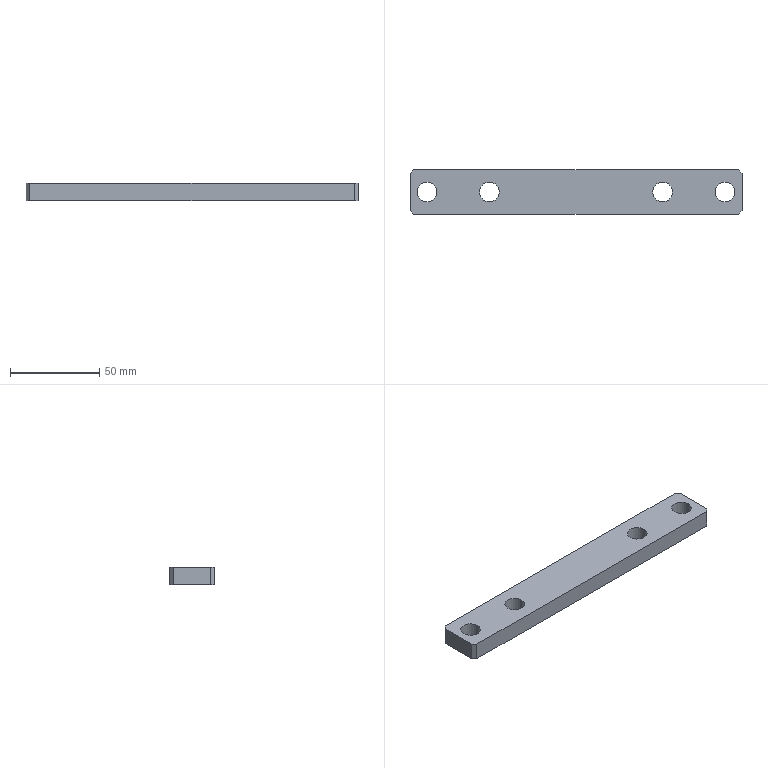Part | STEP file | Pad Plate | 1 solid | 18 faces | box 186 x 25 x 10 mm | volume 42619 mm3 | plane 10 | cylinder 8 | commonest cylinder face diameters 11 x8
STEP:
#1=CARTESIAN_POINT('',(0.,0.,0.));
#2=DIRECTION('',(0.,0.,1.));
#3=DIRECTION('',(1.,0.,0.));
#4=AXIS2_PLACEMENT_3D('',#1,#2,#3);
#5=CARTESIAN_POINT('',(89.,0.,0.));
#6=VERTEX_POINT('',#5);
#7=CARTESIAN_POINT('',(89.,0.,10.));
#8=VERTEX_POINT('',#7);
#9=CARTESIAN_POINT('',(89.,0.,-0.001));
#10=DIRECTION('',(0.,0.,1.));
#11=VECTOR('',#10,1.);
#12=LINE('',#9,#11);
#13=CARTESIAN_POINT('',(83.5,0.,-0.001));
#14=DIRECTION('',(0.,0.,1.));
#15=DIRECTION('',(1.,0.,0.));
#16=AXIS2_PLACEMENT_3D('',#13,#14,#15);
#17=CYLINDRICAL_SURFACE('',#16,5.5);
#18=CARTESIAN_POINT('',(6.283,0.));
#19=DIRECTION('',(0.,1.));
#20=VECTOR('',#19,1.);
#21=LINE('',#18,#20);
#22=(GEOMETRIC_REPRESENTATION_CONTEXT(2)PARAMETRIC_REPRESENTATION_CONTEXT()REPRESENTATION_CONTEXT('',''));
#23=DEFINITIONAL_REPRESENTATION('',(#21),#22);
#24=PCURVE('',#17,#23);
#25=CARTESIAN_POINT('',(83.5,0.,-0.001));
#26=DIRECTION('',(0.,0.,1.));
#27=DIRECTION('',(1.,0.,0.));
#28=AXIS2_PLACEMENT_3D('',#25,#26,#27);
#29=CYLINDRICAL_SURFACE('',#28,5.5);
#30=CARTESIAN_POINT('',(0.,0.));
#31=DIRECTION('',(0.,1.));
#32=VECTOR('',#31,1.);
#33=LINE('',#30,#32);
#34=(GEOMETRIC_REPRESENTATION_CONTEXT(2)PARAMETRIC_REPRESENTATION_CONTEXT()REPRESENTATION_CONTEXT('',''));
#35=DEFINITIONAL_REPRESENTATION('',(#33),#34);
#36=PCURVE('',#29,#35);
#37=SURFACE_CURVE('',#12,(#24,#36),.PCURVE_S1.);
#38=EDGE_CURVE('',#6,#8,#37,.T.);
#39=ORIENTED_EDGE('',*,*,#38,.T.);
#40=CARTESIAN_POINT('',(78.,0.,10.));
#41=VERTEX_POINT('',#40);
#42=CARTESIAN_POINT('',(83.5,0.,10.));
#43=DIRECTION('',(0.,0.,1.));
#44=DIRECTION('',(1.,0.,0.));
#45=AXIS2_PLACEMENT_3D('',#42,#43,#44);
#46=CIRCLE('',#45,5.5);
#47=CARTESIAN_POINT('',(0.,10.001));
#48=DIRECTION('',(1.,0.));
#49=VECTOR('',#48,1.);
#50=LINE('',#47,#49);
#51=(GEOMETRIC_REPRESENTATION_CONTEXT(2)PARAMETRIC_REPRESENTATION_CONTEXT()REPRESENTATION_CONTEXT('',''));
#52=DEFINITIONAL_REPRESENTATION('',(#50),#51);
#53=PCURVE('',#17,#52);
#54=CARTESIAN_POINT('',(0.,0.,10.));
#55=DIRECTION('',(0.,0.,1.));
#56=DIRECTION('',(1.,0.,0.));
#57=AXIS2_PLACEMENT_3D('',#54,#55,#56);
#58=PLANE('',#57);
#59=CARTESIAN_POINT('',(83.5,0.));
#60=DIRECTION('',(1.,0.));
#61=AXIS2_PLACEMENT_2D('',#59,#60);
#62=CIRCLE('',#61,5.5);
#63=(GEOMETRIC_REPRESENTATION_CONTEXT(2)PARAMETRIC_REPRESENTATION_CONTEXT()REPRESENTATION_CONTEXT('',''));
#64=DEFINITIONAL_REPRESENTATION('',(#62),#63);
#65=PCURVE('',#58,#64);
#66=SURFACE_CURVE('',#46,(#53,#65),.PCURVE_S1.);
#67=EDGE_CURVE('',#41,#8,#66,.T.);
#68=ORIENTED_EDGE('',*,*,#67,.F.);
#69=CARTESIAN_POINT('',(78.,0.,0.));
#70=VERTEX_POINT('',#69);
#71=CARTESIAN_POINT('',(78.,0.,-0.001));
#72=DIRECTION('',(0.,0.,1.));
#73=VECTOR('',#72,1.);
#74=LINE('',#71,#73);
#75=CARTESIAN_POINT('',(3.142,0.));
#76=DIRECTION('',(0.,1.));
#77=VECTOR('',#76,1.);
#78=LINE('',#75,#77);
#79=(GEOMETRIC_REPRESENTATION_CONTEXT(2)PARAMETRIC_REPRESENTATION_CONTEXT()REPRESENTATION_CONTEXT('',''));
#80=DEFINITIONAL_REPRESENTATION('',(#78),#79);
#81=PCURVE('',#17,#80);
#82=CARTESIAN_POINT('',(3.142,0.));
#83=DIRECTION('',(0.,1.));
#84=VECTOR('',#83,1.);
#85=LINE('',#82,#84);
#86=(GEOMETRIC_REPRESENTATION_CONTEXT(2)PARAMETRIC_REPRESENTATION_CONTEXT()REPRESENTATION_CONTEXT('',''));
#87=DEFINITIONAL_REPRESENTATION('',(#85),#86);
#88=PCURVE('',#29,#87);
#89=SURFACE_CURVE('',#74,(#81,#88),.PCURVE_S1.);
#90=EDGE_CURVE('',#70,#41,#89,.T.);
#91=ORIENTED_EDGE('',*,*,#90,.F.);
#92=CARTESIAN_POINT('',(83.5,0.,0.));
#93=DIRECTION('',(0.,0.,-1.));
#94=DIRECTION('',(1.,0.,0.));
#95=AXIS2_PLACEMENT_3D('',#92,#93,#94);
#96=CIRCLE('',#95,5.5);
#97=CARTESIAN_POINT('',(6.283,0.001));
#98=DIRECTION('',(-1.,0.));
#99=VECTOR('',#98,1.);
#100=LINE('',#97,#99);
#101=(GEOMETRIC_REPRESENTATION_CONTEXT(2)PARAMETRIC_REPRESENTATION_CONTEXT()REPRESENTATION_CONTEXT('',''));
#102=DEFINITIONAL_REPRESENTATION('',(#100),#101);
#103=PCURVE('',#17,#102);
#104=CARTESIAN_POINT('',(0.,0.,0.));
#105=DIRECTION('',(0.,0.,1.));
#106=DIRECTION('',(1.,0.,0.));
#107=AXIS2_PLACEMENT_3D('',#104,#105,#106);
#108=PLANE('',#107);
#109=CARTESIAN_POINT('',(89.,0.));
#110=CARTESIAN_POINT('',(89.,-9.526));
#111=CARTESIAN_POINT('',(80.75,-4.763));
#112=CARTESIAN_POINT('',(72.5,0.));
#113=CARTESIAN_POINT('',(80.75,4.763));
#114=CARTESIAN_POINT('',(89.,9.526));
#115=CARTESIAN_POINT('',(89.,0.));
#116=(BOUNDED_CURVE()B_SPLINE_CURVE(2,(#109,#110,#111,#112,#113,#114,#115),.UNSPECIFIED.,.T.,.F.)B_SPLINE_CURVE_WITH_KNOTS((1,2,2,2,2,1),(-2.094,0.,2.094,4.189,6.283,8.378),.UNSPECIFIED.)CURVE()GEOMETRIC_REPRESENTATION_ITEM()RATIONAL_B_SPLINE_CURVE((1.,0.5,1.,0.5,1.,0.5,1.))REPRESENTATION_ITEM(''));
#117=(GEOMETRIC_REPRESENTATION_CONTEXT(2)PARAMETRIC_REPRESENTATION_CONTEXT()REPRESENTATION_CONTEXT('',''));
#118=DEFINITIONAL_REPRESENTATION('',(#116),#117);
#119=PCURVE('',#108,#118);
#120=SURFACE_CURVE('',#96,(#103,#119),.PCURVE_S1.);
#121=EDGE_CURVE('',#6,#70,#120,.T.);
#122=ORIENTED_EDGE('',*,*,#121,.F.);
#123=EDGE_LOOP('',(#39,#68,#91,#122));
#124=FACE_BOUND('',#123,.F.);
#125=ADVANCED_FACE('',(#124),#17,.F.);
#126=CARTESIAN_POINT('',(54.,0.,0.));
#127=VERTEX_POINT('',#126);
#128=CARTESIAN_POINT('',(54.,0.,10.));
#129=VERTEX_POINT('',#128);
#130=CARTESIAN_POINT('',(54.,0.,-0.001));
#131=DIRECTION('',(0.,0.,1.));
#132=VECTOR('',#131,1.);
#133=LINE('',#130,#132);
#134=CARTESIAN_POINT('',(48.5,0.,-0.001));
#135=DIRECTION('',(0.,0.,1.));
#136=DIRECTION('',(1.,0.,0.));
#137=AXIS2_PLACEMENT_3D('',#134,#135,#136);
#138=CYLINDRICAL_SURFACE('',#137,5.5);
#139=CARTESIAN_POINT('',(6.283,0.));
#140=DIRECTION('',(0.,1.));
#141=VECTOR('',#140,1.);
#142=LINE('',#139,#141);
#143=(GEOMETRIC_REPRESENTATION_CONTEXT(2)PARAMETRIC_REPRESENTATION_CONTEXT()REPRESENTATION_CONTEXT('',''));
#144=DEFINITIONAL_REPRESENTATION('',(#142),#143);
#145=PCURVE('',#138,#144);
#146=CARTESIAN_POINT('',(48.5,0.,-0.001));
#147=DIRECTION('',(0.,0.,1.));
#148=DIRECTION('',(1.,0.,0.));
#149=AXIS2_PLACEMENT_3D('',#146,#147,#148);
#150=CYLINDRICAL_SURFACE('',#149,5.5);
#151=CARTESIAN_POINT('',(0.,0.));
#152=DIRECTION('',(0.,1.));
#153=VECTOR('',#152,1.);
#154=LINE('',#151,#153);
#155=(GEOMETRIC_REPRESENTATION_CONTEXT(2)PARAMETRIC_REPRESENTATION_CONTEXT()REPRESENTATION_CONTEXT('',''));
#156=DEFINITIONAL_REPRESENTATION('',(#154),#155);
#157=PCURVE('',#150,#156);
#158=SURFACE_CURVE('',#133,(#145,#157),.PCURVE_S1.);
#159=EDGE_CURVE('',#127,#129,#158,.T.);
#160=ORIENTED_EDGE('',*,*,#159,.T.);
#161=CARTESIAN_POINT('',(43.,0.,10.));
#162=VERTEX_POINT('',#161);
#163=CARTESIAN_POINT('',(48.5,0.,10.));
#164=DIRECTION('',(0.,0.,1.));
#165=DIRECTION('',(1.,0.,0.));
#166=AXIS2_PLACEMENT_3D('',#163,#164,#165);
#167=CIRCLE('',#166,5.5);
#168=CARTESIAN_POINT('',(0.,10.001));
#169=DIRECTION('',(1.,0.));
#170=VECTOR('',#169,1.);
#171=LINE('',#168,#170);
#172=(GEOMETRIC_REPRESENTATION_CONTEXT(2)PARAMETRIC_REPRESENTATION_CONTEXT()REPRESENTATION_CONTEXT('',''));
#173=DEFINITIONAL_REPRESENTATION('',(#171),#172);
#174=PCURVE('',#138,#173);
#175=CARTESIAN_POINT('',(48.5,0.));
#176=DIRECTION('',(1.,0.));
#177=AXIS2_PLACEMENT_2D('',#175,#176);
#178=CIRCLE('',#177,5.5);
#179=(GEOMETRIC_REPRESENTATION_CONTEXT(2)PARAMETRIC_REPRESENTATION_CONTEXT()REPRESENTATION_CONTEXT('',''));
#180=DEFINITIONAL_REPRESENTATION('',(#178),#179);
#181=PCURVE('',#58,#180);
#182=SURFACE_CURVE('',#167,(#174,#181),.PCURVE_S1.);
#183=EDGE_CURVE('',#162,#129,#182,.T.);
#184=ORIENTED_EDGE('',*,*,#183,.F.);
#185=CARTESIAN_POINT('',(43.,0.,0.));
#186=VERTEX_POINT('',#185);
#187=CARTESIAN_POINT('',(43.,0.,-0.001));
#188=DIRECTION('',(0.,0.,1.));
#189=VECTOR('',#188,1.);
#190=LINE('',#187,#189);
#191=CARTESIAN_POINT('',(3.142,0.));
#192=DIRECTION('',(0.,1.));
#193=VECTOR('',#192,1.);
#194=LINE('',#191,#193);
#195=(GEOMETRIC_REPRESENTATION_CONTEXT(2)PARAMETRIC_REPRESENTATION_CONTEXT()REPRESENTATION_CONTEXT('',''));
#196=DEFINITIONAL_REPRESENTATION('',(#194),#195);
#197=PCURVE('',#138,#196);
#198=CARTESIAN_POINT('',(3.142,0.));
#199=DIRECTION('',(0.,1.));
#200=VECTOR('',#199,1.);
#201=LINE('',#198,#200);
#202=(GEOMETRIC_REPRESENTATION_CONTEXT(2)PARAMETRIC_REPRESENTATION_CONTEXT()REPRESENTATION_CONTEXT('',''));
#203=DEFINITIONAL_REPRESENTATION('',(#201),#202);
#204=PCURVE('',#150,#203);
#205=SURFACE_CURVE('',#190,(#197,#204),.PCURVE_S1.);
#206=EDGE_CURVE('',#186,#162,#205,.T.);
#207=ORIENTED_EDGE('',*,*,#206,.F.);
#208=CARTESIAN_POINT('',(48.5,0.,0.));
#209=DIRECTION('',(0.,0.,-1.));
#210=DIRECTION('',(1.,0.,0.));
#211=AXIS2_PLACEMENT_3D('',#208,#209,#210);
#212=CIRCLE('',#211,5.5);
#213=CARTESIAN_POINT('',(6.283,0.001));
#214=DIRECTION('',(-1.,0.));
#215=VECTOR('',#214,1.);
#216=LINE('',#213,#215);
#217=(GEOMETRIC_REPRESENTATION_CONTEXT(2)PARAMETRIC_REPRESENTATION_CONTEXT()REPRESENTATION_CONTEXT('',''));
#218=DEFINITIONAL_REPRESENTATION('',(#216),#217);
#219=PCURVE('',#138,#218);
#220=CARTESIAN_POINT('',(54.,0.));
#221=CARTESIAN_POINT('',(54.,-9.526));
#222=CARTESIAN_POINT('',(45.75,-4.763));
#223=CARTESIAN_POINT('',(37.5,0.));
#224=CARTESIAN_POINT('',(45.75,4.763));
#225=CARTESIAN_POINT('',(54.,9.526));
#226=CARTESIAN_POINT('',(54.,0.));
#227=(BOUNDED_CURVE()B_SPLINE_CURVE(2,(#220,#221,#222,#223,#224,#225,#226),.UNSPECIFIED.,.T.,.F.)B_SPLINE_CURVE_WITH_KNOTS((1,2,2,2,2,1),(-2.094,0.,2.094,4.189,6.283,8.378),.UNSPECIFIED.)CURVE()GEOMETRIC_REPRESENTATION_ITEM()RATIONAL_B_SPLINE_CURVE((1.,0.5,1.,0.5,1.,0.5,1.))REPRESENTATION_ITEM(''));
#228=(GEOMETRIC_REPRESENTATION_CONTEXT(2)PARAMETRIC_REPRESENTATION_CONTEXT()REPRESENTATION_CONTEXT('',''));
#229=DEFINITIONAL_REPRESENTATION('',(#227),#228);
#230=PCURVE('',#108,#229);
#231=SURFACE_CURVE('',#212,(#219,#230),.PCURVE_S1.);
#232=EDGE_CURVE('',#127,#186,#231,.T.);
#233=ORIENTED_EDGE('',*,*,#232,.F.);
#234=EDGE_LOOP('',(#160,#184,#207,#233));
#235=FACE_BOUND('',#234,.F.);
#236=ADVANCED_FACE('',(#235),#138,.F.);
#237=CARTESIAN_POINT('',(-43.,0.,0.));
#238=VERTEX_POINT('',#237);
#239=CARTESIAN_POINT('',(-43.,0.,10.));
#240=VERTEX_POINT('',#239);
#241=CARTESIAN_POINT('',(-43.,0.,-0.001));
#242=DIRECTION('',(0.,0.,1.));
#243=VECTOR('',#242,1.);
#244=LINE('',#241,#243);
#245=CARTESIAN_POINT('',(-48.5,0.,-0.001));
#246=DIRECTION('',(0.,0.,1.));
#247=DIRECTION('',(1.,0.,0.));
#248=AXIS2_PLACEMENT_3D('',#245,#246,#247);
#249=CYLINDRICAL_SURFACE('',#248,5.5);
#250=CARTESIAN_POINT('',(6.283,0.));
#251=DIRECTION('',(0.,1.));
#252=VECTOR('',#251,1.);
#253=LINE('',#250,#252);
#254=(GEOMETRIC_REPRESENTATION_CONTEXT(2)PARAMETRIC_REPRESENTATION_CONTEXT()REPRESENTATION_CONTEXT('',''));
#255=DEFINITIONAL_REPRESENTATION('',(#253),#254);
#256=PCURVE('',#249,#255);
#257=CARTESIAN_POINT('',(-48.5,0.,-0.001));
#258=DIRECTION('',(0.,0.,1.));
#259=DIRECTION('',(1.,0.,0.));
#260=AXIS2_PLACEMENT_3D('',#257,#258,#259);
#261=CYLINDRICAL_SURFACE('',#260,5.5);
#262=CARTESIAN_POINT('',(0.,0.));
#263=DIRECTION('',(0.,1.));
#264=VECTOR('',#263,1.);
#265=LINE('',#262,#264);
#266=(GEOMETRIC_REPRESENTATION_CONTEXT(2)PARAMETRIC_REPRESENTATION_CONTEXT()REPRESENTATION_CONTEXT('',''));
#267=DEFINITIONAL_REPRESENTATION('',(#265),#266);
#268=PCURVE('',#261,#267);
#269=SURFACE_CURVE('',#244,(#256,#268),.PCURVE_S1.);
#270=EDGE_CURVE('',#238,#240,#269,.T.);
#271=ORIENTED_EDGE('',*,*,#270,.T.);
#272=CARTESIAN_POINT('',(-54.,0.,10.));
#273=VERTEX_POINT('',#272);
#274=CARTESIAN_POINT('',(-48.5,0.,10.));
#275=DIRECTION('',(0.,0.,1.));
#276=DIRECTION('',(1.,0.,0.));
#277=AXIS2_PLACEMENT_3D('',#274,#275,#276);
#278=CIRCLE('',#277,5.5);
#279=CARTESIAN_POINT('',(0.,10.001));
#280=DIRECTION('',(1.,0.));
#281=VECTOR('',#280,1.);
#282=LINE('',#279,#281);
#283=(GEOMETRIC_REPRESENTATION_CONTEXT(2)PARAMETRIC_REPRESENTATION_CONTEXT()REPRESENTATION_CONTEXT('',''));
#284=DEFINITIONAL_REPRESENTATION('',(#282),#283);
#285=PCURVE('',#249,#284);
#286=CARTESIAN_POINT('',(-48.5,0.));
#287=DIRECTION('',(1.,0.));
#288=AXIS2_PLACEMENT_2D('',#286,#287);
#289=CIRCLE('',#288,5.5);
#290=(GEOMETRIC_REPRESENTATION_CONTEXT(2)PARAMETRIC_REPRESENTATION_CONTEXT()REPRESENTATION_CONTEXT('',''));
#291=DEFINITIONAL_REPRESENTATION('',(#289),#290);
#292=PCURVE('',#58,#291);
#293=SURFACE_CURVE('',#278,(#285,#292),.PCURVE_S1.);
#294=EDGE_CURVE('',#273,#240,#293,.T.);
#295=ORIENTED_EDGE('',*,*,#294,.F.);
#296=CARTESIAN_POINT('',(-54.,0.,0.));
#297=VERTEX_POINT('',#296);
#298=CARTESIAN_POINT('',(-54.,0.,-0.001));
#299=DIRECTION('',(0.,0.,1.));
#300=VECTOR('',#299,1.);
#301=LINE('',#298,#300);
#302=CARTESIAN_POINT('',(3.142,0.));
#303=DIRECTION('',(0.,1.));
#304=VECTOR('',#303,1.);
#305=LINE('',#302,#304);
#306=(GEOMETRIC_REPRESENTATION_CONTEXT(2)PARAMETRIC_REPRESENTATION_CONTEXT()REPRESENTATION_CONTEXT('',''));
#307=DEFINITIONAL_REPRESENTATION('',(#305),#306);
#308=PCURVE('',#249,#307);
#309=CARTESIAN_POINT('',(3.142,0.));
#310=DIRECTION('',(0.,1.));
#311=VECTOR('',#310,1.);
#312=LINE('',#309,#311);
#313=(GEOMETRIC_REPRESENTATION_CONTEXT(2)PARAMETRIC_REPRESENTATION_CONTEXT()REPRESENTATION_CONTEXT('',''));
#314=DEFINITIONAL_REPRESENTATION('',(#312),#313);
#315=PCURVE('',#261,#314);
#316=SURFACE_CURVE('',#301,(#308,#315),.PCURVE_S1.);
#317=EDGE_CURVE('',#297,#273,#316,.T.);
#318=ORIENTED_EDGE('',*,*,#317,.F.);
#319=CARTESIAN_POINT('',(-48.5,0.,0.));
#320=DIRECTION('',(0.,0.,-1.));
#321=DIRECTION('',(1.,0.,0.));
#322=AXIS2_PLACEMENT_3D('',#319,#320,#321);
#323=CIRCLE('',#322,5.5);
#324=CARTESIAN_POINT('',(6.283,0.001));
#325=DIRECTION('',(-1.,0.));
#326=VECTOR('',#325,1.);
#327=LINE('',#324,#326);
#328=(GEOMETRIC_REPRESENTATION_CONTEXT(2)PARAMETRIC_REPRESENTATION_CONTEXT()REPRESENTATION_CONTEXT('',''));
#329=DEFINITIONAL_REPRESENTATION('',(#327),#328);
#330=PCURVE('',#249,#329);
#331=CARTESIAN_POINT('',(-43.,0.));
#332=CARTESIAN_POINT('',(-43.,-9.526));
#333=CARTESIAN_POINT('',(-51.25,-4.763));
#334=CARTESIAN_POINT('',(-59.5,0.));
#335=CARTESIAN_POINT('',(-51.25,4.763));
#336=CARTESIAN_POINT('',(-43.,9.526));
#337=CARTESIAN_POINT('',(-43.,0.));
#338=(BOUNDED_CURVE()B_SPLINE_CURVE(2,(#331,#332,#333,#334,#335,#336,#337),.UNSPECIFIED.,.T.,.F.)B_SPLINE_CURVE_WITH_KNOTS((1,2,2,2,2,1),(-2.094,0.,2.094,4.189,6.283,8.378),.UNSPECIFIED.)CURVE()GEOMETRIC_REPRESENTATION_ITEM()RATIONAL_B_SPLINE_CURVE((1.,0.5,1.,0.5,1.,0.5,1.))REPRESENTATION_ITEM(''));
#339=(GEOMETRIC_REPRESENTATION_CONTEXT(2)PARAMETRIC_REPRESENTATION_CONTEXT()REPRESENTATION_CONTEXT('',''));
#340=DEFINITIONAL_REPRESENTATION('',(#338),#339);
#341=PCURVE('',#108,#340);
#342=SURFACE_CURVE('',#323,(#330,#341),.PCURVE_S1.);
#343=EDGE_CURVE('',#238,#297,#342,.T.);
#344=ORIENTED_EDGE('',*,*,#343,.F.);
#345=EDGE_LOOP('',(#271,#295,#318,#344));
#346=FACE_BOUND('',#345,.F.);
#347=ADVANCED_FACE('',(#346),#249,.F.);
#348=CARTESIAN_POINT('',(-78.,0.,0.));
#349=VERTEX_POINT('',#348);
#350=CARTESIAN_POINT('',(-78.,0.,10.));
#351=VERTEX_POINT('',#350);
#352=CARTESIAN_POINT('',(-78.,0.,-0.001));
#353=DIRECTION('',(0.,0.,1.));
#354=VECTOR('',#353,1.);
#355=LINE('',#352,#354);
#356=CARTESIAN_POINT('',(-83.5,0.,-0.001));
#357=DIRECTION('',(0.,0.,1.));
#358=DIRECTION('',(1.,0.,0.));
#359=AXIS2_PLACEMENT_3D('',#356,#357,#358);
#360=CYLINDRICAL_SURFACE('',#359,5.5);
#361=CARTESIAN_POINT('',(6.283,0.));
#362=DIRECTION('',(0.,1.));
#363=VECTOR('',#362,1.);
#364=LINE('',#361,#363);
#365=(GEOMETRIC_REPRESENTATION_CONTEXT(2)PARAMETRIC_REPRESENTATION_CONTEXT()REPRESENTATION_CONTEXT('',''));
#366=DEFINITIONAL_REPRESENTATION('',(#364),#365);
#367=PCURVE('',#360,#366);
#368=CARTESIAN_POINT('',(-83.5,0.,-0.001));
#369=DIRECTION('',(0.,0.,1.));
#370=DIRECTION('',(1.,0.,0.));
#371=AXIS2_PLACEMENT_3D('',#368,#369,#370);
#372=CYLINDRICAL_SURFACE('',#371,5.5);
#373=CARTESIAN_POINT('',(0.,0.));
#374=DIRECTION('',(0.,1.));
#375=VECTOR('',#374,1.);
#376=LINE('',#373,#375);
#377=(GEOMETRIC_REPRESENTATION_CONTEXT(2)PARAMETRIC_REPRESENTATION_CONTEXT()REPRESENTATION_CONTEXT('',''));
#378=DEFINITIONAL_REPRESENTATION('',(#376),#377);
#379=PCURVE('',#372,#378);
#380=SURFACE_CURVE('',#355,(#367,#379),.PCURVE_S1.);
#381=EDGE_CURVE('',#349,#351,#380,.T.);
#382=ORIENTED_EDGE('',*,*,#381,.T.);
#383=CARTESIAN_POINT('',(-89.,0.,10.));
#384=VERTEX_POINT('',#383);
#385=CARTESIAN_POINT('',(-83.5,0.,10.));
#386=DIRECTION('',(0.,0.,1.));
#387=DIRECTION('',(1.,0.,0.));
#388=AXIS2_PLACEMENT_3D('',#385,#386,#387);
#389=CIRCLE('',#388,5.5);
#390=CARTESIAN_POINT('',(0.,10.001));
#391=DIRECTION('',(1.,0.));
#392=VECTOR('',#391,1.);
#393=LINE('',#390,#392);
#394=(GEOMETRIC_REPRESENTATION_CONTEXT(2)PARAMETRIC_REPRESENTATION_CONTEXT()REPRESENTATION_CONTEXT('',''));
#395=DEFINITIONAL_REPRESENTATION('',(#393),#394);
#396=PCURVE('',#360,#395);
#397=CARTESIAN_POINT('',(-83.5,0.));
#398=DIRECTION('',(1.,0.));
#399=AXIS2_PLACEMENT_2D('',#397,#398);
#400=CIRCLE('',#399,5.5);
#401=(GEOMETRIC_REPRESENTATION_CONTEXT(2)PARAMETRIC_REPRESENTATION_CONTEXT()REPRESENTATION_CONTEXT('',''));
#402=DEFINITIONAL_REPRESENTATION('',(#400),#401);
#403=PCURVE('',#58,#402);
#404=SURFACE_CURVE('',#389,(#396,#403),.PCURVE_S1.);
#405=EDGE_CURVE('',#384,#351,#404,.T.);
#406=ORIENTED_EDGE('',*,*,#405,.F.);
#407=CARTESIAN_POINT('',(-89.,0.,0.));
#408=VERTEX_POINT('',#407);
#409=CARTESIAN_POINT('',(-89.,0.,-0.001));
#410=DIRECTION('',(0.,0.,1.));
#411=VECTOR('',#410,1.);
#412=LINE('',#409,#411);
#413=CARTESIAN_POINT('',(3.142,0.));
#414=DIRECTION('',(0.,1.));
#415=VECTOR('',#414,1.);
#416=LINE('',#413,#415);
#417=(GEOMETRIC_REPRESENTATION_CONTEXT(2)PARAMETRIC_REPRESENTATION_CONTEXT()REPRESENTATION_CONTEXT('',''));
#418=DEFINITIONAL_REPRESENTATION('',(#416),#417);
#419=PCURVE('',#360,#418);
#420=CARTESIAN_POINT('',(3.142,0.));
#421=DIRECTION('',(0.,1.));
#422=VECTOR('',#421,1.);
#423=LINE('',#420,#422);
#424=(GEOMETRIC_REPRESENTATION_CONTEXT(2)PARAMETRIC_REPRESENTATION_CONTEXT()REPRESENTATION_CONTEXT('',''));
#425=DEFINITIONAL_REPRESENTATION('',(#423),#424);
#426=PCURVE('',#372,#425);
#427=SURFACE_CURVE('',#412,(#419,#426),.PCURVE_S1.);
#428=EDGE_CURVE('',#408,#384,#427,.T.);
#429=ORIENTED_EDGE('',*,*,#428,.F.);
#430=CARTESIAN_POINT('',(-83.5,0.,0.));
#431=DIRECTION('',(0.,0.,-1.));
#432=DIRECTION('',(1.,0.,0.));
#433=AXIS2_PLACEMENT_3D('',#430,#431,#432);
#434=CIRCLE('',#433,5.5);
#435=CARTESIAN_POINT('',(6.283,0.001));
#436=DIRECTION('',(-1.,0.));
#437=VECTOR('',#436,1.);
#438=LINE('',#435,#437);
#439=(GEOMETRIC_REPRESENTATION_CONTEXT(2)PARAMETRIC_REPRESENTATION_CONTEXT()REPRESENTATION_CONTEXT('',''));
#440=DEFINITIONAL_REPRESENTATION('',(#438),#439);
#441=PCURVE('',#360,#440);
#442=CARTESIAN_POINT('',(-78.,0.));
#443=CARTESIAN_POINT('',(-78.,-9.526));
#444=CARTESIAN_POINT('',(-86.25,-4.763));
#445=CARTESIAN_POINT('',(-94.5,0.));
#446=CARTESIAN_POINT('',(-86.25,4.763));
#447=CARTESIAN_POINT('',(-78.,9.526));
#448=CARTESIAN_POINT('',(-78.,0.));
#449=(BOUNDED_CURVE()B_SPLINE_CURVE(2,(#442,#443,#444,#445,#446,#447,#448),.UNSPECIFIED.,.T.,.F.)B_SPLINE_CURVE_WITH_KNOTS((1,2,2,2,2,1),(-2.094,0.,2.094,4.189,6.283,8.378),.UNSPECIFIED.)CURVE()GEOMETRIC_REPRESENTATION_ITEM()RATIONAL_B_SPLINE_CURVE((1.,0.5,1.,0.5,1.,0.5,1.))REPRESENTATION_ITEM(''));
#450=(GEOMETRIC_REPRESENTATION_CONTEXT(2)PARAMETRIC_REPRESENTATION_CONTEXT()REPRESENTATION_CONTEXT('',''));
#451=DEFINITIONAL_REPRESENTATION('',(#449),#450);
#452=PCURVE('',#108,#451);
#453=SURFACE_CURVE('',#434,(#441,#452),.PCURVE_S1.);
#454=EDGE_CURVE('',#349,#408,#453,.T.);
#455=ORIENTED_EDGE('',*,*,#454,.F.);
#456=EDGE_LOOP('',(#382,#406,#429,#455));
#457=FACE_BOUND('',#456,.F.);
#458=ADVANCED_FACE('',(#457),#360,.F.);
#459=CARTESIAN_POINT('',(93.,-10.5,10.));
#460=VERTEX_POINT('',#459);
#461=CARTESIAN_POINT('',(93.,10.5,10.));
#462=VERTEX_POINT('',#461);
#463=CARTESIAN_POINT('',(93.,12.5,10.));
#464=DIRECTION('',(0.,1.,0.));
#465=VECTOR('',#464,1.);
#466=LINE('',#463,#465);
#467=CARTESIAN_POINT('',(93.,12.5,10.));
#468=DIRECTION('',(-1.,0.,0.));
#469=DIRECTION('',(0.,0.,1.));
#470=AXIS2_PLACEMENT_3D('',#467,#468,#469);
#471=PLANE('',#470);
#472=CARTESIAN_POINT('',(0.,0.));
#473=DIRECTION('',(0.,1.));
#474=VECTOR('',#473,1.);
#475=LINE('',#472,#474);
#476=(GEOMETRIC_REPRESENTATION_CONTEXT(2)PARAMETRIC_REPRESENTATION_CONTEXT()REPRESENTATION_CONTEXT('',''));
#477=DEFINITIONAL_REPRESENTATION('',(#475),#476);
#478=PCURVE('',#471,#477);
#479=CARTESIAN_POINT('',(93.,12.5));
#480=DIRECTION('',(0.,1.));
#481=VECTOR('',#480,1.);
#482=LINE('',#479,#481);
#483=(GEOMETRIC_REPRESENTATION_CONTEXT(2)PARAMETRIC_REPRESENTATION_CONTEXT()REPRESENTATION_CONTEXT('',''));
#484=DEFINITIONAL_REPRESENTATION('',(#482),#483);
#485=PCURVE('',#58,#484);
#486=SURFACE_CURVE('',#466,(#478,#485),.PCURVE_S1.);
#487=EDGE_CURVE('',#460,#462,#486,.T.);
#488=ORIENTED_EDGE('',*,*,#487,.F.);
#489=CARTESIAN_POINT('',(93.,-10.5,0.));
#490=VERTEX_POINT('',#489);
#491=CARTESIAN_POINT('',(93.,-10.5,10.));
#492=DIRECTION('',(0.,0.,-1.));
#493=VECTOR('',#492,1.);
#494=LINE('',#491,#493);
#495=CARTESIAN_POINT('',(0.,-23.));
#496=DIRECTION('',(-1.,0.));
#497=VECTOR('',#496,1.);
#498=LINE('',#495,#497);
#499=(GEOMETRIC_REPRESENTATION_CONTEXT(2)PARAMETRIC_REPRESENTATION_CONTEXT()REPRESENTATION_CONTEXT('',''));
#500=DEFINITIONAL_REPRESENTATION('',(#498),#499);
#501=PCURVE('',#471,#500);
#502=CARTESIAN_POINT('',(93.,-10.5,10.));
#503=DIRECTION('',(-0.7071,0.7071,0.));
#504=DIRECTION('',(0.,0.,-1.));
#505=AXIS2_PLACEMENT_3D('',#502,#503,#504);
#506=PLANE('',#505);
#507=CARTESIAN_POINT('',(0.,0.));
#508=DIRECTION('',(1.,0.));
#509=VECTOR('',#508,1.);
#510=LINE('',#507,#509);
#511=(GEOMETRIC_REPRESENTATION_CONTEXT(2)PARAMETRIC_REPRESENTATION_CONTEXT()REPRESENTATION_CONTEXT('',''));
#512=DEFINITIONAL_REPRESENTATION('',(#510),#511);
#513=PCURVE('',#506,#512);
#514=SURFACE_CURVE('',#494,(#501,#513),.PCURVE_S1.);
#515=EDGE_CURVE('',#460,#490,#514,.T.);
#516=ORIENTED_EDGE('',*,*,#515,.T.);
#517=CARTESIAN_POINT('',(93.,10.5,0.));
#518=VERTEX_POINT('',#517);
#519=CARTESIAN_POINT('',(93.,12.5,0.));
#520=DIRECTION('',(0.,1.,0.));
#521=VECTOR('',#520,1.);
#522=LINE('',#519,#521);
#523=CARTESIAN_POINT('',(-10.,0.));
#524=DIRECTION('',(0.,1.));
#525=VECTOR('',#524,1.);
#526=LINE('',#523,#525);
#527=(GEOMETRIC_REPRESENTATION_CONTEXT(2)PARAMETRIC_REPRESENTATION_CONTEXT()REPRESENTATION_CONTEXT('',''));
#528=DEFINITIONAL_REPRESENTATION('',(#526),#527);
#529=PCURVE('',#471,#528);
#530=CARTESIAN_POINT('',(93.,12.5));
#531=DIRECTION('',(0.,1.));
#532=VECTOR('',#531,1.);
#533=LINE('',#530,#532);
#534=(GEOMETRIC_REPRESENTATION_CONTEXT(2)PARAMETRIC_REPRESENTATION_CONTEXT()REPRESENTATION_CONTEXT('',''));
#535=DEFINITIONAL_REPRESENTATION('',(#533),#534);
#536=PCURVE('',#108,#535);
#537=SURFACE_CURVE('',#522,(#529,#536),.PCURVE_S1.);
#538=EDGE_CURVE('',#490,#518,#537,.T.);
#539=ORIENTED_EDGE('',*,*,#538,.T.);
#540=CARTESIAN_POINT('',(93.,10.5,10.));
#541=DIRECTION('',(0.,0.,1.));
#542=VECTOR('',#541,1.);
#543=LINE('',#540,#542);
#544=CARTESIAN_POINT('',(0.,-2.));
#545=DIRECTION('',(1.,0.));
#546=VECTOR('',#545,1.);
#547=LINE('',#544,#546);
#548=(GEOMETRIC_REPRESENTATION_CONTEXT(2)PARAMETRIC_REPRESENTATION_CONTEXT()REPRESENTATION_CONTEXT('',''));
#549=DEFINITIONAL_REPRESENTATION('',(#547),#548);
#550=PCURVE('',#471,#549);
#551=CARTESIAN_POINT('',(91.,12.5,10.));
#552=DIRECTION('',(-0.7071,-0.7071,0.));
#553=DIRECTION('',(0.,0.,-1.));
#554=AXIS2_PLACEMENT_3D('',#551,#552,#553);
#555=PLANE('',#554);
#556=CARTESIAN_POINT('',(0.,2.828));
#557=DIRECTION('',(-1.,0.));
#558=VECTOR('',#557,1.);
#559=LINE('',#556,#558);
#560=(GEOMETRIC_REPRESENTATION_CONTEXT(2)PARAMETRIC_REPRESENTATION_CONTEXT()REPRESENTATION_CONTEXT('',''));
#561=DEFINITIONAL_REPRESENTATION('',(#559),#560);
#562=PCURVE('',#555,#561);
#563=SURFACE_CURVE('',#543,(#550,#562),.PCURVE_S1.);
#564=EDGE_CURVE('',#518,#462,#563,.T.);
#565=ORIENTED_EDGE('',*,*,#564,.T.);
#566=EDGE_LOOP('',(#488,#516,#539,#565));
#567=FACE_BOUND('',#566,.T.);
#568=ADVANCED_FACE('',(#567),#471,.F.);
#569=CARTESIAN_POINT('',(91.,12.5,10.));
#570=VERTEX_POINT('',#569);
#571=CARTESIAN_POINT('',(-91.,12.5,10.));
#572=VERTEX_POINT('',#571);
#573=CARTESIAN_POINT('',(-93.,12.5,10.));
#574=DIRECTION('',(-1.,0.,0.));
#575=VECTOR('',#574,1.);
#576=LINE('',#573,#575);
#577=CARTESIAN_POINT('',(-93.,12.5,10.));
#578=DIRECTION('',(0.,-1.,0.));
#579=DIRECTION('',(0.,0.,-1.));
#580=AXIS2_PLACEMENT_3D('',#577,#578,#579);
#581=PLANE('',#580);
#582=CARTESIAN_POINT('',(0.,0.));
#583=DIRECTION('',(0.,-1.));
#584=VECTOR('',#583,1.);
#585=LINE('',#582,#584);
#586=(GEOMETRIC_REPRESENTATION_CONTEXT(2)PARAMETRIC_REPRESENTATION_CONTEXT()REPRESENTATION_CONTEXT('',''));
#587=DEFINITIONAL_REPRESENTATION('',(#585),#586);
#588=PCURVE('',#581,#587);
#589=CARTESIAN_POINT('',(-93.,12.5));
#590=DIRECTION('',(-1.,0.));
#591=VECTOR('',#590,1.);
#592=LINE('',#589,#591);
#593=(GEOMETRIC_REPRESENTATION_CONTEXT(2)PARAMETRIC_REPRESENTATION_CONTEXT()REPRESENTATION_CONTEXT('',''));
#594=DEFINITIONAL_REPRESENTATION('',(#592),#593);
#595=PCURVE('',#58,#594);
#596=SURFACE_CURVE('',#576,(#588,#595),.PCURVE_S1.);
#597=EDGE_CURVE('',#570,#572,#596,.T.);
#598=ORIENTED_EDGE('',*,*,#597,.F.);
#599=CARTESIAN_POINT('',(91.,12.5,0.));
#600=VERTEX_POINT('',#599);
#601=CARTESIAN_POINT('',(91.,12.5,10.));
#602=DIRECTION('',(0.,0.,-1.));
#603=VECTOR('',#602,1.);
#604=LINE('',#601,#603);
#605=CARTESIAN_POINT('',(0.,184.));
#606=DIRECTION('',(1.,0.));
#607=VECTOR('',#606,1.);
#608=LINE('',#605,#607);
#609=(GEOMETRIC_REPRESENTATION_CONTEXT(2)PARAMETRIC_REPRESENTATION_CONTEXT()REPRESENTATION_CONTEXT('',''));
#610=DEFINITIONAL_REPRESENTATION('',(#608),#609);
#611=PCURVE('',#581,#610);
#612=CARTESIAN_POINT('',(0.,0.));
#613=DIRECTION('',(1.,0.));
#614=VECTOR('',#613,1.);
#615=LINE('',#612,#614);
#616=(GEOMETRIC_REPRESENTATION_CONTEXT(2)PARAMETRIC_REPRESENTATION_CONTEXT()REPRESENTATION_CONTEXT('',''));
#617=DEFINITIONAL_REPRESENTATION('',(#615),#616);
#618=PCURVE('',#555,#617);
#619=SURFACE_CURVE('',#604,(#611,#618),.PCURVE_S1.);
#620=EDGE_CURVE('',#570,#600,#619,.T.);
#621=ORIENTED_EDGE('',*,*,#620,.T.);
#622=CARTESIAN_POINT('',(-91.,12.5,0.));
#623=VERTEX_POINT('',#622);
#624=CARTESIAN_POINT('',(-93.,12.5,0.));
#625=DIRECTION('',(-1.,0.,0.));
#626=VECTOR('',#625,1.);
#627=LINE('',#624,#626);
#628=CARTESIAN_POINT('',(10.,0.));
#629=DIRECTION('',(0.,-1.));
#630=VECTOR('',#629,1.);
#631=LINE('',#628,#630);
#632=(GEOMETRIC_REPRESENTATION_CONTEXT(2)PARAMETRIC_REPRESENTATION_CONTEXT()REPRESENTATION_CONTEXT('',''));
#633=DEFINITIONAL_REPRESENTATION('',(#631),#632);
#634=PCURVE('',#581,#633);
#635=CARTESIAN_POINT('',(-93.,12.5));
#636=DIRECTION('',(-1.,0.));
#637=VECTOR('',#636,1.);
#638=LINE('',#635,#637);
#639=(GEOMETRIC_REPRESENTATION_CONTEXT(2)PARAMETRIC_REPRESENTATION_CONTEXT()REPRESENTATION_CONTEXT('',''));
#640=DEFINITIONAL_REPRESENTATION('',(#638),#639);
#641=PCURVE('',#108,#640);
#642=SURFACE_CURVE('',#627,(#634,#641),.PCURVE_S1.);
#643=EDGE_CURVE('',#600,#623,#642,.T.);
#644=ORIENTED_EDGE('',*,*,#643,.T.);
#645=CARTESIAN_POINT('',(-91.,12.5,10.));
#646=DIRECTION('',(0.,0.,1.));
#647=VECTOR('',#646,1.);
#648=LINE('',#645,#647);
#649=CARTESIAN_POINT('',(0.,2.));
#650=DIRECTION('',(-1.,0.));
#651=VECTOR('',#650,1.);
#652=LINE('',#649,#651);
#653=(GEOMETRIC_REPRESENTATION_CONTEXT(2)PARAMETRIC_REPRESENTATION_CONTEXT()REPRESENTATION_CONTEXT('',''));
#654=DEFINITIONAL_REPRESENTATION('',(#652),#653);
#655=PCURVE('',#581,#654);
#656=CARTESIAN_POINT('',(-93.,10.5,10.));
#657=DIRECTION('',(0.7071,-0.7071,0.));
#658=DIRECTION('',(0.,0.,-1.));
#659=AXIS2_PLACEMENT_3D('',#656,#657,#658);
#660=PLANE('',#659);
#661=CARTESIAN_POINT('',(0.,2.828));
#662=DIRECTION('',(-1.,0.));
#663=VECTOR('',#662,1.);
#664=LINE('',#661,#663);
#665=(GEOMETRIC_REPRESENTATION_CONTEXT(2)PARAMETRIC_REPRESENTATION_CONTEXT()REPRESENTATION_CONTEXT('',''));
#666=DEFINITIONAL_REPRESENTATION('',(#664),#665);
#667=PCURVE('',#660,#666);
#668=SURFACE_CURVE('',#648,(#655,#667),.PCURVE_S1.);
#669=EDGE_CURVE('',#623,#572,#668,.T.);
#670=ORIENTED_EDGE('',*,*,#669,.T.);
#671=EDGE_LOOP('',(#598,#621,#644,#670));
#672=FACE_BOUND('',#671,.T.);
#673=ADVANCED_FACE('',(#672),#581,.F.);
#674=CARTESIAN_POINT('',(-93.,10.5,10.));
#675=VERTEX_POINT('',#674);
#676=CARTESIAN_POINT('',(-93.,-10.5,10.));
#677=VERTEX_POINT('',#676);
#678=CARTESIAN_POINT('',(-93.,12.5,10.));
#679=DIRECTION('',(0.,-1.,0.));
#680=VECTOR('',#679,1.);
#681=LINE('',#678,#680);
#682=CARTESIAN_POINT('',(-93.,12.5,10.));
#683=DIRECTION('',(1.,0.,0.));
#684=DIRECTION('',(0.,0.,-1.));
#685=AXIS2_PLACEMENT_3D('',#682,#683,#684);
#686=PLANE('',#685);
#687=CARTESIAN_POINT('',(0.,0.));
#688=DIRECTION('',(0.,-1.));
#689=VECTOR('',#688,1.);
#690=LINE('',#687,#689);
#691=(GEOMETRIC_REPRESENTATION_CONTEXT(2)PARAMETRIC_REPRESENTATION_CONTEXT()REPRESENTATION_CONTEXT('',''));
#692=DEFINITIONAL_REPRESENTATION('',(#690),#691);
#693=PCURVE('',#686,#692);
#694=CARTESIAN_POINT('',(-93.,12.5));
#695=DIRECTION('',(0.,-1.));
#696=VECTOR('',#695,1.);
#697=LINE('',#694,#696);
#698=(GEOMETRIC_REPRESENTATION_CONTEXT(2)PARAMETRIC_REPRESENTATION_CONTEXT()REPRESENTATION_CONTEXT('',''));
#699=DEFINITIONAL_REPRESENTATION('',(#697),#698);
#700=PCURVE('',#58,#699);
#701=SURFACE_CURVE('',#681,(#693,#700),.PCURVE_S1.);
#702=EDGE_CURVE('',#675,#677,#701,.T.);
#703=ORIENTED_EDGE('',*,*,#702,.F.);
#704=CARTESIAN_POINT('',(-93.,10.5,0.));
#705=VERTEX_POINT('',#704);
#706=CARTESIAN_POINT('',(-93.,10.5,10.));
#707=DIRECTION('',(0.,0.,-1.));
#708=VECTOR('',#707,1.);
#709=LINE('',#706,#708);
#710=CARTESIAN_POINT('',(0.,-2.));
#711=DIRECTION('',(1.,0.));
#712=VECTOR('',#711,1.);
#713=LINE('',#710,#712);
#714=(GEOMETRIC_REPRESENTATION_CONTEXT(2)PARAMETRIC_REPRESENTATION_CONTEXT()REPRESENTATION_CONTEXT('',''));
#715=DEFINITIONAL_REPRESENTATION('',(#713),#714);
#716=PCURVE('',#686,#715);
#717=CARTESIAN_POINT('',(0.,0.));
#718=DIRECTION('',(1.,0.));
#719=VECTOR('',#718,1.);
#720=LINE('',#717,#719);
#721=(GEOMETRIC_REPRESENTATION_CONTEXT(2)PARAMETRIC_REPRESENTATION_CONTEXT()REPRESENTATION_CONTEXT('',''));
#722=DEFINITIONAL_REPRESENTATION('',(#720),#721);
#723=PCURVE('',#660,#722);
#724=SURFACE_CURVE('',#709,(#716,#723),.PCURVE_S1.);
#725=EDGE_CURVE('',#675,#705,#724,.T.);
#726=ORIENTED_EDGE('',*,*,#725,.T.);
#727=CARTESIAN_POINT('',(-93.,-10.5,0.));
#728=VERTEX_POINT('',#727);
#729=CARTESIAN_POINT('',(-93.,12.5,0.));
#730=DIRECTION('',(0.,-1.,0.));
#731=VECTOR('',#730,1.);
#732=LINE('',#729,#731);
#733=CARTESIAN_POINT('',(10.,0.));
#734=DIRECTION('',(0.,-1.));
#735=VECTOR('',#734,1.);
#736=LINE('',#733,#735);
#737=(GEOMETRIC_REPRESENTATION_CONTEXT(2)PARAMETRIC_REPRESENTATION_CONTEXT()REPRESENTATION_CONTEXT('',''));
#738=DEFINITIONAL_REPRESENTATION('',(#736),#737);
#739=PCURVE('',#686,#738);
#740=CARTESIAN_POINT('',(-93.,12.5));
#741=DIRECTION('',(0.,-1.));
#742=VECTOR('',#741,1.);
#743=LINE('',#740,#742);
#744=(GEOMETRIC_REPRESENTATION_CONTEXT(2)PARAMETRIC_REPRESENTATION_CONTEXT()REPRESENTATION_CONTEXT('',''));
#745=DEFINITIONAL_REPRESENTATION('',(#743),#744);
#746=PCURVE('',#108,#745);
#747=SURFACE_CURVE('',#732,(#739,#746),.PCURVE_S1.);
#748=EDGE_CURVE('',#705,#728,#747,.T.);
#749=ORIENTED_EDGE('',*,*,#748,.T.);
#750=CARTESIAN_POINT('',(-93.,-10.5,10.));
#751=DIRECTION('',(0.,0.,1.));
#752=VECTOR('',#751,1.);
#753=LINE('',#750,#752);
#754=CARTESIAN_POINT('',(0.,-23.));
#755=DIRECTION('',(-1.,0.));
#756=VECTOR('',#755,1.);
#757=LINE('',#754,#756);
#758=(GEOMETRIC_REPRESENTATION_CONTEXT(2)PARAMETRIC_REPRESENTATION_CONTEXT()REPRESENTATION_CONTEXT('',''));
#759=DEFINITIONAL_REPRESENTATION('',(#757),#758);
#760=PCURVE('',#686,#759);
#761=CARTESIAN_POINT('',(-91.,-12.5,10.));
#762=DIRECTION('',(0.7071,0.7071,0.));
#763=DIRECTION('',(0.,0.,-1.));
#764=AXIS2_PLACEMENT_3D('',#761,#762,#763);
#765=PLANE('',#764);
#766=CARTESIAN_POINT('',(0.,2.828));
#767=DIRECTION('',(-1.,0.));
#768=VECTOR('',#767,1.);
#769=LINE('',#766,#768);
#770=(GEOMETRIC_REPRESENTATION_CONTEXT(2)PARAMETRIC_REPRESENTATION_CONTEXT()REPRESENTATION_CONTEXT('',''));
#771=DEFINITIONAL_REPRESENTATION('',(#769),#770);
#772=PCURVE('',#765,#771);
#773=SURFACE_CURVE('',#753,(#760,#772),.PCURVE_S1.);
#774=EDGE_CURVE('',#728,#677,#773,.T.);
#775=ORIENTED_EDGE('',*,*,#774,.T.);
#776=EDGE_LOOP('',(#703,#726,#749,#775));
#777=FACE_BOUND('',#776,.T.);
#778=ADVANCED_FACE('',(#777),#686,.F.);
#779=CARTESIAN_POINT('',(-91.,-12.5,0.));
#780=VERTEX_POINT('',#779);
#781=CARTESIAN_POINT('',(91.,-12.5,0.));
#782=VERTEX_POINT('',#781);
#783=CARTESIAN_POINT('',(-93.,-12.5,0.));
#784=DIRECTION('',(1.,0.,0.));
#785=VECTOR('',#784,1.);
#786=LINE('',#783,#785);
#787=CARTESIAN_POINT('',(-93.,-12.5,10.));
#788=DIRECTION('',(0.,1.,0.));
#789=DIRECTION('',(0.,0.,1.));
#790=AXIS2_PLACEMENT_3D('',#787,#788,#789);
#791=PLANE('',#790);
#792=CARTESIAN_POINT('',(-10.,0.));
#793=DIRECTION('',(0.,1.));
#794=VECTOR('',#793,1.);
#795=LINE('',#792,#794);
#796=(GEOMETRIC_REPRESENTATION_CONTEXT(2)PARAMETRIC_REPRESENTATION_CONTEXT()REPRESENTATION_CONTEXT('',''));
#797=DEFINITIONAL_REPRESENTATION('',(#795),#796);
#798=PCURVE('',#791,#797);
#799=CARTESIAN_POINT('',(-93.,-12.5));
#800=DIRECTION('',(1.,0.));
#801=VECTOR('',#800,1.);
#802=LINE('',#799,#801);
#803=(GEOMETRIC_REPRESENTATION_CONTEXT(2)PARAMETRIC_REPRESENTATION_CONTEXT()REPRESENTATION_CONTEXT('',''));
#804=DEFINITIONAL_REPRESENTATION('',(#802),#803);
#805=PCURVE('',#108,#804);
#806=SURFACE_CURVE('',#786,(#798,#805),.PCURVE_S1.);
#807=EDGE_CURVE('',#780,#782,#806,.T.);
#808=ORIENTED_EDGE('',*,*,#807,.T.);
#809=CARTESIAN_POINT('',(91.,-12.5,10.));
#810=VERTEX_POINT('',#809);
#811=CARTESIAN_POINT('',(91.,-12.5,10.));
#812=DIRECTION('',(0.,0.,1.));
#813=VECTOR('',#812,1.);
#814=LINE('',#811,#813);
#815=CARTESIAN_POINT('',(0.,184.));
#816=DIRECTION('',(1.,0.));
#817=VECTOR('',#816,1.);
#818=LINE('',#815,#817);
#819=(GEOMETRIC_REPRESENTATION_CONTEXT(2)PARAMETRIC_REPRESENTATION_CONTEXT()REPRESENTATION_CONTEXT('',''));
#820=DEFINITIONAL_REPRESENTATION('',(#818),#819);
#821=PCURVE('',#791,#820);
#822=CARTESIAN_POINT('',(0.,2.828));
#823=DIRECTION('',(-1.,0.));
#824=VECTOR('',#823,1.);
#825=LINE('',#822,#824);
#826=(GEOMETRIC_REPRESENTATION_CONTEXT(2)PARAMETRIC_REPRESENTATION_CONTEXT()REPRESENTATION_CONTEXT('',''));
#827=DEFINITIONAL_REPRESENTATION('',(#825),#826);
#828=PCURVE('',#506,#827);
#829=SURFACE_CURVE('',#814,(#821,#828),.PCURVE_S1.);
#830=EDGE_CURVE('',#782,#810,#829,.T.);
#831=ORIENTED_EDGE('',*,*,#830,.T.);
#832=CARTESIAN_POINT('',(-91.,-12.5,10.));
#833=VERTEX_POINT('',#832);
#834=CARTESIAN_POINT('',(-93.,-12.5,10.));
#835=DIRECTION('',(1.,0.,0.));
#836=VECTOR('',#835,1.);
#837=LINE('',#834,#836);
#838=CARTESIAN_POINT('',(0.,0.));
#839=DIRECTION('',(0.,1.));
#840=VECTOR('',#839,1.);
#841=LINE('',#838,#840);
#842=(GEOMETRIC_REPRESENTATION_CONTEXT(2)PARAMETRIC_REPRESENTATION_CONTEXT()REPRESENTATION_CONTEXT('',''));
#843=DEFINITIONAL_REPRESENTATION('',(#841),#842);
#844=PCURVE('',#791,#843);
#845=CARTESIAN_POINT('',(-93.,-12.5));
#846=DIRECTION('',(1.,0.));
#847=VECTOR('',#846,1.);
#848=LINE('',#845,#847);
#849=(GEOMETRIC_REPRESENTATION_CONTEXT(2)PARAMETRIC_REPRESENTATION_CONTEXT()REPRESENTATION_CONTEXT('',''));
#850=DEFINITIONAL_REPRESENTATION('',(#848),#849);
#851=PCURVE('',#58,#850);
#852=SURFACE_CURVE('',#837,(#844,#851),.PCURVE_S1.);
#853=EDGE_CURVE('',#833,#810,#852,.T.);
#854=ORIENTED_EDGE('',*,*,#853,.F.);
#855=CARTESIAN_POINT('',(-91.,-12.5,10.));
#856=DIRECTION('',(0.,0.,-1.));
#857=VECTOR('',#856,1.);
#858=LINE('',#855,#857);
#859=CARTESIAN_POINT('',(0.,2.));
#860=DIRECTION('',(-1.,0.));
#861=VECTOR('',#860,1.);
#862=LINE('',#859,#861);
#863=(GEOMETRIC_REPRESENTATION_CONTEXT(2)PARAMETRIC_REPRESENTATION_CONTEXT()REPRESENTATION_CONTEXT('',''));
#864=DEFINITIONAL_REPRESENTATION('',(#862),#863);
#865=PCURVE('',#791,#864);
#866=CARTESIAN_POINT('',(0.,0.));
#867=DIRECTION('',(1.,0.));
#868=VECTOR('',#867,1.);
#869=LINE('',#866,#868);
#870=(GEOMETRIC_REPRESENTATION_CONTEXT(2)PARAMETRIC_REPRESENTATION_CONTEXT()REPRESENTATION_CONTEXT('',''));
#871=DEFINITIONAL_REPRESENTATION('',(#869),#870);
#872=PCURVE('',#765,#871);
#873=SURFACE_CURVE('',#858,(#865,#872),.PCURVE_S1.);
#874=EDGE_CURVE('',#833,#780,#873,.T.);
#875=ORIENTED_EDGE('',*,*,#874,.T.);
#876=EDGE_LOOP('',(#808,#831,#854,#875));
#877=FACE_BOUND('',#876,.T.);
#878=ADVANCED_FACE('',(#877),#791,.F.);
#879=CARTESIAN_POINT('',(83.5,0.,10.));
#880=DIRECTION('',(0.,0.,1.));
#881=DIRECTION('',(1.,0.,0.));
#882=AXIS2_PLACEMENT_3D('',#879,#880,#881);
#883=CIRCLE('',#882,5.5);
#884=CARTESIAN_POINT('',(83.5,0.));
#885=DIRECTION('',(1.,0.));
#886=AXIS2_PLACEMENT_2D('',#884,#885);
#887=CIRCLE('',#886,5.5);
#888=(GEOMETRIC_REPRESENTATION_CONTEXT(2)PARAMETRIC_REPRESENTATION_CONTEXT()REPRESENTATION_CONTEXT('',''));
#889=DEFINITIONAL_REPRESENTATION('',(#887),#888);
#890=PCURVE('',#58,#889);
#891=CARTESIAN_POINT('',(0.,10.001));
#892=DIRECTION('',(1.,0.));
#893=VECTOR('',#892,1.);
#894=LINE('',#891,#893);
#895=(GEOMETRIC_REPRESENTATION_CONTEXT(2)PARAMETRIC_REPRESENTATION_CONTEXT()REPRESENTATION_CONTEXT('',''));
#896=DEFINITIONAL_REPRESENTATION('',(#894),#895);
#897=PCURVE('',#29,#896);
#898=SURFACE_CURVE('',#883,(#890,#897),.PCURVE_S1.);
#899=EDGE_CURVE('',#8,#41,#898,.T.);
#900=ORIENTED_EDGE('',*,*,#899,.F.);
#901=ORIENTED_EDGE('',*,*,#67,.F.);
#902=EDGE_LOOP('',(#900,#901));
#903=FACE_BOUND('',#902,.T.);
#904=CARTESIAN_POINT('',(48.5,0.,10.));
#905=DIRECTION('',(0.,0.,1.));
#906=DIRECTION('',(1.,0.,0.));
#907=AXIS2_PLACEMENT_3D('',#904,#905,#906);
#908=CIRCLE('',#907,5.5);
#909=CARTESIAN_POINT('',(48.5,0.));
#910=DIRECTION('',(1.,0.));
#911=AXIS2_PLACEMENT_2D('',#909,#910);
#912=CIRCLE('',#911,5.5);
#913=(GEOMETRIC_REPRESENTATION_CONTEXT(2)PARAMETRIC_REPRESENTATION_CONTEXT()REPRESENTATION_CONTEXT('',''));
#914=DEFINITIONAL_REPRESENTATION('',(#912),#913);
#915=PCURVE('',#58,#914);
#916=CARTESIAN_POINT('',(0.,10.001));
#917=DIRECTION('',(1.,0.));
#918=VECTOR('',#917,1.);
#919=LINE('',#916,#918);
#920=(GEOMETRIC_REPRESENTATION_CONTEXT(2)PARAMETRIC_REPRESENTATION_CONTEXT()REPRESENTATION_CONTEXT('',''));
#921=DEFINITIONAL_REPRESENTATION('',(#919),#920);
#922=PCURVE('',#150,#921);
#923=SURFACE_CURVE('',#908,(#915,#922),.PCURVE_S1.);
#924=EDGE_CURVE('',#129,#162,#923,.T.);
#925=ORIENTED_EDGE('',*,*,#924,.F.);
#926=ORIENTED_EDGE('',*,*,#183,.F.);
#927=EDGE_LOOP('',(#925,#926));
#928=FACE_BOUND('',#927,.T.);
#929=CARTESIAN_POINT('',(-48.5,0.,10.));
#930=DIRECTION('',(0.,0.,1.));
#931=DIRECTION('',(1.,0.,0.));
#932=AXIS2_PLACEMENT_3D('',#929,#930,#931);
#933=CIRCLE('',#932,5.5);
#934=CARTESIAN_POINT('',(-48.5,0.));
#935=DIRECTION('',(1.,0.));
#936=AXIS2_PLACEMENT_2D('',#934,#935);
#937=CIRCLE('',#936,5.5);
#938=(GEOMETRIC_REPRESENTATION_CONTEXT(2)PARAMETRIC_REPRESENTATION_CONTEXT()REPRESENTATION_CONTEXT('',''));
#939=DEFINITIONAL_REPRESENTATION('',(#937),#938);
#940=PCURVE('',#58,#939);
#941=CARTESIAN_POINT('',(0.,10.001));
#942=DIRECTION('',(1.,0.));
#943=VECTOR('',#942,1.);
#944=LINE('',#941,#943);
#945=(GEOMETRIC_REPRESENTATION_CONTEXT(2)PARAMETRIC_REPRESENTATION_CONTEXT()REPRESENTATION_CONTEXT('',''));
#946=DEFINITIONAL_REPRESENTATION('',(#944),#945);
#947=PCURVE('',#261,#946);
#948=SURFACE_CURVE('',#933,(#940,#947),.PCURVE_S1.);
#949=EDGE_CURVE('',#240,#273,#948,.T.);
#950=ORIENTED_EDGE('',*,*,#949,.F.);
#951=ORIENTED_EDGE('',*,*,#294,.F.);
#952=EDGE_LOOP('',(#950,#951));
#953=FACE_BOUND('',#952,.T.);
#954=CARTESIAN_POINT('',(-83.5,0.,10.));
#955=DIRECTION('',(0.,0.,1.));
#956=DIRECTION('',(1.,0.,0.));
#957=AXIS2_PLACEMENT_3D('',#954,#955,#956);
#958=CIRCLE('',#957,5.5);
#959=CARTESIAN_POINT('',(-83.5,0.));
#960=DIRECTION('',(1.,0.));
#961=AXIS2_PLACEMENT_2D('',#959,#960);
#962=CIRCLE('',#961,5.5);
#963=(GEOMETRIC_REPRESENTATION_CONTEXT(2)PARAMETRIC_REPRESENTATION_CONTEXT()REPRESENTATION_CONTEXT('',''));
#964=DEFINITIONAL_REPRESENTATION('',(#962),#963);
#965=PCURVE('',#58,#964);
#966=CARTESIAN_POINT('',(0.,10.001));
#967=DIRECTION('',(1.,0.));
#968=VECTOR('',#967,1.);
#969=LINE('',#966,#968);
#970=(GEOMETRIC_REPRESENTATION_CONTEXT(2)PARAMETRIC_REPRESENTATION_CONTEXT()REPRESENTATION_CONTEXT('',''));
#971=DEFINITIONAL_REPRESENTATION('',(#969),#970);
#972=PCURVE('',#372,#971);
#973=SURFACE_CURVE('',#958,(#965,#972),.PCURVE_S1.);
#974=EDGE_CURVE('',#351,#384,#973,.T.);
#975=ORIENTED_EDGE('',*,*,#974,.F.);
#976=ORIENTED_EDGE('',*,*,#405,.F.);
#977=EDGE_LOOP('',(#975,#976));
#978=FACE_BOUND('',#977,.T.);
#979=ORIENTED_EDGE('',*,*,#853,.T.);
#980=CARTESIAN_POINT('',(51.75,-51.75,10.));
#981=DIRECTION('',(0.7071,0.7071,0.));
#982=VECTOR('',#981,1.);
#983=LINE('',#980,#982);
#984=CARTESIAN_POINT('',(51.75,-51.75));
#985=DIRECTION('',(0.7071,0.7071));
#986=VECTOR('',#985,1.);
#987=LINE('',#984,#986);
#988=(GEOMETRIC_REPRESENTATION_CONTEXT(2)PARAMETRIC_REPRESENTATION_CONTEXT()REPRESENTATION_CONTEXT('',''));
#989=DEFINITIONAL_REPRESENTATION('',(#987),#988);
#990=PCURVE('',#58,#989);
#991=CARTESIAN_POINT('',(0.,58.336));
#992=DIRECTION('',(0.,-1.));
#993=VECTOR('',#992,1.);
#994=LINE('',#991,#993);
#995=(GEOMETRIC_REPRESENTATION_CONTEXT(2)PARAMETRIC_REPRESENTATION_CONTEXT()REPRESENTATION_CONTEXT('',''));
#996=DEFINITIONAL_REPRESENTATION('',(#994),#995);
#997=PCURVE('',#506,#996);
#998=SURFACE_CURVE('',#983,(#990,#997),.PCURVE_S1.);
#999=EDGE_CURVE('',#810,#460,#998,.T.);
#1000=ORIENTED_EDGE('',*,*,#999,.T.);
#1001=ORIENTED_EDGE('',*,*,#487,.T.);
#1002=CARTESIAN_POINT('',(51.75,51.75,10.));
#1003=DIRECTION('',(-0.7071,0.7071,0.));
#1004=VECTOR('',#1003,1.);
#1005=LINE('',#1002,#1004);
#1006=CARTESIAN_POINT('',(51.75,51.75));
#1007=DIRECTION('',(-0.7071,0.7071));
#1008=VECTOR('',#1007,1.);
#1009=LINE('',#1006,#1008);
#1010=(GEOMETRIC_REPRESENTATION_CONTEXT(2)PARAMETRIC_REPRESENTATION_CONTEXT()REPRESENTATION_CONTEXT('',''));
#1011=DEFINITIONAL_REPRESENTATION('',(#1009),#1010);
#1012=PCURVE('',#58,#1011);
#1013=CARTESIAN_POINT('',(0.,-55.508));
#1014=DIRECTION('',(0.,-1.));
#1015=VECTOR('',#1014,1.);
#1016=LINE('',#1013,#1015);
#1017=(GEOMETRIC_REPRESENTATION_CONTEXT(2)PARAMETRIC_REPRESENTATION_CONTEXT()REPRESENTATION_CONTEXT('',''));
#1018=DEFINITIONAL_REPRESENTATION('',(#1016),#1017);
#1019=PCURVE('',#555,#1018);
#1020=SURFACE_CURVE('',#1005,(#1012,#1019),.PCURVE_S1.);
#1021=EDGE_CURVE('',#462,#570,#1020,.T.);
#1022=ORIENTED_EDGE('',*,*,#1021,.T.);
#1023=ORIENTED_EDGE('',*,*,#597,.T.);
#1024=CARTESIAN_POINT('',(-51.75,51.75,10.));
#1025=DIRECTION('',(-0.7071,-0.7071,0.));
#1026=VECTOR('',#1025,1.);
#1027=LINE('',#1024,#1026);
#1028=CARTESIAN_POINT('',(-51.75,51.75));
#1029=DIRECTION('',(-0.7071,-0.7071));
#1030=VECTOR('',#1029,1.);
#1031=LINE('',#1028,#1030);
#1032=(GEOMETRIC_REPRESENTATION_CONTEXT(2)PARAMETRIC_REPRESENTATION_CONTEXT()REPRESENTATION_CONTEXT('',''));
#1033=DEFINITIONAL_REPRESENTATION('',(#1031),#1032);
#1034=PCURVE('',#58,#1033);
#1035=CARTESIAN_POINT('',(0.,58.336));
#1036=DIRECTION('',(0.,-1.));
#1037=VECTOR('',#1036,1.);
#1038=LINE('',#1035,#1037);
#1039=(GEOMETRIC_REPRESENTATION_CONTEXT(2)PARAMETRIC_REPRESENTATION_CONTEXT()REPRESENTATION_CONTEXT('',''));
#1040=DEFINITIONAL_REPRESENTATION('',(#1038),#1039);
#1041=PCURVE('',#660,#1040);
#1042=SURFACE_CURVE('',#1027,(#1034,#1041),.PCURVE_S1.);
#1043=EDGE_CURVE('',#572,#675,#1042,.T.);
#1044=ORIENTED_EDGE('',*,*,#1043,.T.);
#1045=ORIENTED_EDGE('',*,*,#702,.T.);
#1046=CARTESIAN_POINT('',(-51.75,-51.75,10.));
#1047=DIRECTION('',(0.7071,-0.7071,0.));
#1048=VECTOR('',#1047,1.);
#1049=LINE('',#1046,#1048);
#1050=CARTESIAN_POINT('',(-51.75,-51.75));
#1051=DIRECTION('',(0.7071,-0.7071));
#1052=VECTOR('',#1051,1.);
#1053=LINE('',#1050,#1052);
#1054=(GEOMETRIC_REPRESENTATION_CONTEXT(2)PARAMETRIC_REPRESENTATION_CONTEXT()REPRESENTATION_CONTEXT('',''));
#1055=DEFINITIONAL_REPRESENTATION('',(#1053),#1054);
#1056=PCURVE('',#58,#1055);
#1057=CARTESIAN_POINT('',(0.,-55.508));
#1058=DIRECTION('',(0.,-1.));
#1059=VECTOR('',#1058,1.);
#1060=LINE('',#1057,#1059);
#1061=(GEOMETRIC_REPRESENTATION_CONTEXT(2)PARAMETRIC_REPRESENTATION_CONTEXT()REPRESENTATION_CONTEXT('',''));
#1062=DEFINITIONAL_REPRESENTATION('',(#1060),#1061);
#1063=PCURVE('',#765,#1062);
#1064=SURFACE_CURVE('',#1049,(#1056,#1063),.PCURVE_S1.);
#1065=EDGE_CURVE('',#677,#833,#1064,.T.);
#1066=ORIENTED_EDGE('',*,*,#1065,.T.);
#1067=EDGE_LOOP('',(#979,#1000,#1001,#1022,#1023,#1044,#1045,#1066));
#1068=FACE_BOUND('',#1067,.T.);
#1069=ADVANCED_FACE('',(#903,#928,#953,#978,#1068),#58,.T.);
#1070=ORIENTED_EDGE('',*,*,#121,.F.);
#1071=CARTESIAN_POINT('',(83.5,0.,0.));
#1072=DIRECTION('',(0.,0.,-1.));
#1073=DIRECTION('',(1.,0.,0.));
#1074=AXIS2_PLACEMENT_3D('',#1071,#1072,#1073);
#1075=CIRCLE('',#1074,5.5);
#1076=CARTESIAN_POINT('',(89.,0.));
#1077=CARTESIAN_POINT('',(89.,-9.526));
#1078=CARTESIAN_POINT('',(80.75,-4.763));
#1079=CARTESIAN_POINT('',(72.5,0.));
#1080=CARTESIAN_POINT('',(80.75,4.763));
#1081=CARTESIAN_POINT('',(89.,9.526));
#1082=CARTESIAN_POINT('',(89.,0.));
#1083=(BOUNDED_CURVE()B_SPLINE_CURVE(2,(#1076,#1077,#1078,#1079,#1080,#1081,#1082),.UNSPECIFIED.,.T.,.F.)B_SPLINE_CURVE_WITH_KNOTS((1,2,2,2,2,1),(-2.094,0.,2.094,4.189,6.283,8.378),.UNSPECIFIED.)CURVE()GEOMETRIC_REPRESENTATION_ITEM()RATIONAL_B_SPLINE_CURVE((1.,0.5,1.,0.5,1.,0.5,1.))REPRESENTATION_ITEM(''));
#1084=(GEOMETRIC_REPRESENTATION_CONTEXT(2)PARAMETRIC_REPRESENTATION_CONTEXT()REPRESENTATION_CONTEXT('',''));
#1085=DEFINITIONAL_REPRESENTATION('',(#1083),#1084);
#1086=PCURVE('',#108,#1085);
#1087=CARTESIAN_POINT('',(6.283,0.001));
#1088=DIRECTION('',(-1.,0.));
#1089=VECTOR('',#1088,1.);
#1090=LINE('',#1087,#1089);
#1091=(GEOMETRIC_REPRESENTATION_CONTEXT(2)PARAMETRIC_REPRESENTATION_CONTEXT()REPRESENTATION_CONTEXT('',''));
#1092=DEFINITIONAL_REPRESENTATION('',(#1090),#1091);
#1093=PCURVE('',#29,#1092);
#1094=SURFACE_CURVE('',#1075,(#1086,#1093),.PCURVE_S1.);
#1095=EDGE_CURVE('',#70,#6,#1094,.T.);
#1096=ORIENTED_EDGE('',*,*,#1095,.F.);
#1097=EDGE_LOOP('',(#1070,#1096));
#1098=FACE_BOUND('',#1097,.T.);
#1099=ORIENTED_EDGE('',*,*,#232,.F.);
#1100=CARTESIAN_POINT('',(48.5,0.,0.));
#1101=DIRECTION('',(0.,0.,-1.));
#1102=DIRECTION('',(1.,0.,0.));
#1103=AXIS2_PLACEMENT_3D('',#1100,#1101,#1102);
#1104=CIRCLE('',#1103,5.5);
#1105=CARTESIAN_POINT('',(54.,0.));
#1106=CARTESIAN_POINT('',(54.,-9.526));
#1107=CARTESIAN_POINT('',(45.75,-4.763));
#1108=CARTESIAN_POINT('',(37.5,0.));
#1109=CARTESIAN_POINT('',(45.75,4.763));
#1110=CARTESIAN_POINT('',(54.,9.526));
#1111=CARTESIAN_POINT('',(54.,0.));
#1112=(BOUNDED_CURVE()B_SPLINE_CURVE(2,(#1105,#1106,#1107,#1108,#1109,#1110,#1111),.UNSPECIFIED.,.T.,.F.)B_SPLINE_CURVE_WITH_KNOTS((1,2,2,2,2,1),(-2.094,0.,2.094,4.189,6.283,8.378),.UNSPECIFIED.)CURVE()GEOMETRIC_REPRESENTATION_ITEM()RATIONAL_B_SPLINE_CURVE((1.,0.5,1.,0.5,1.,0.5,1.))REPRESENTATION_ITEM(''));
#1113=(GEOMETRIC_REPRESENTATION_CONTEXT(2)PARAMETRIC_REPRESENTATION_CONTEXT()REPRESENTATION_CONTEXT('',''));
#1114=DEFINITIONAL_REPRESENTATION('',(#1112),#1113);
#1115=PCURVE('',#108,#1114);
#1116=CARTESIAN_POINT('',(6.283,0.001));
#1117=DIRECTION('',(-1.,0.));
#1118=VECTOR('',#1117,1.);
#1119=LINE('',#1116,#1118);
#1120=(GEOMETRIC_REPRESENTATION_CONTEXT(2)PARAMETRIC_REPRESENTATION_CONTEXT()REPRESENTATION_CONTEXT('',''));
#1121=DEFINITIONAL_REPRESENTATION('',(#1119),#1120);
#1122=PCURVE('',#150,#1121);
#1123=SURFACE_CURVE('',#1104,(#1115,#1122),.PCURVE_S1.);
#1124=EDGE_CURVE('',#186,#127,#1123,.T.);
#1125=ORIENTED_EDGE('',*,*,#1124,.F.);
#1126=EDGE_LOOP('',(#1099,#1125));
#1127=FACE_BOUND('',#1126,.T.);
#1128=ORIENTED_EDGE('',*,*,#343,.F.);
#1129=CARTESIAN_POINT('',(-48.5,0.,0.));
#1130=DIRECTION('',(0.,0.,-1.));
#1131=DIRECTION('',(1.,0.,0.));
#1132=AXIS2_PLACEMENT_3D('',#1129,#1130,#1131);
#1133=CIRCLE('',#1132,5.5);
#1134=CARTESIAN_POINT('',(-43.,0.));
#1135=CARTESIAN_POINT('',(-43.,-9.526));
#1136=CARTESIAN_POINT('',(-51.25,-4.763));
#1137=CARTESIAN_POINT('',(-59.5,0.));
#1138=CARTESIAN_POINT('',(-51.25,4.763));
#1139=CARTESIAN_POINT('',(-43.,9.526));
#1140=CARTESIAN_POINT('',(-43.,0.));
#1141=(BOUNDED_CURVE()B_SPLINE_CURVE(2,(#1134,#1135,#1136,#1137,#1138,#1139,#1140),.UNSPECIFIED.,.T.,.F.)B_SPLINE_CURVE_WITH_KNOTS((1,2,2,2,2,1),(-2.094,0.,2.094,4.189,6.283,8.378),.UNSPECIFIED.)CURVE()GEOMETRIC_REPRESENTATION_ITEM()RATIONAL_B_SPLINE_CURVE((1.,0.5,1.,0.5,1.,0.5,1.))REPRESENTATION_ITEM(''));
#1142=(GEOMETRIC_REPRESENTATION_CONTEXT(2)PARAMETRIC_REPRESENTATION_CONTEXT()REPRESENTATION_CONTEXT('',''));
#1143=DEFINITIONAL_REPRESENTATION('',(#1141),#1142);
#1144=PCURVE('',#108,#1143);
#1145=CARTESIAN_POINT('',(6.283,0.001));
#1146=DIRECTION('',(-1.,0.));
#1147=VECTOR('',#1146,1.);
#1148=LINE('',#1145,#1147);
#1149=(GEOMETRIC_REPRESENTATION_CONTEXT(2)PARAMETRIC_REPRESENTATION_CONTEXT()REPRESENTATION_CONTEXT('',''));
#1150=DEFINITIONAL_REPRESENTATION('',(#1148),#1149);
#1151=PCURVE('',#261,#1150);
#1152=SURFACE_CURVE('',#1133,(#1144,#1151),.PCURVE_S1.);
#1153=EDGE_CURVE('',#297,#238,#1152,.T.);
#1154=ORIENTED_EDGE('',*,*,#1153,.F.);
#1155=EDGE_LOOP('',(#1128,#1154));
#1156=FACE_BOUND('',#1155,.T.);
#1157=ORIENTED_EDGE('',*,*,#454,.F.);
#1158=CARTESIAN_POINT('',(-83.5,0.,0.));
#1159=DIRECTION('',(0.,0.,-1.));
#1160=DIRECTION('',(1.,0.,0.));
#1161=AXIS2_PLACEMENT_3D('',#1158,#1159,#1160);
#1162=CIRCLE('',#1161,5.5);
#1163=CARTESIAN_POINT('',(-78.,0.));
#1164=CARTESIAN_POINT('',(-78.,-9.526));
#1165=CARTESIAN_POINT('',(-86.25,-4.763));
#1166=CARTESIAN_POINT('',(-94.5,0.));
#1167=CARTESIAN_POINT('',(-86.25,4.763));
#1168=CARTESIAN_POINT('',(-78.,9.526));
#1169=CARTESIAN_POINT('',(-78.,0.));
#1170=(BOUNDED_CURVE()B_SPLINE_CURVE(2,(#1163,#1164,#1165,#1166,#1167,#1168,#1169),.UNSPECIFIED.,.T.,.F.)B_SPLINE_CURVE_WITH_KNOTS((1,2,2,2,2,1),(-2.094,0.,2.094,4.189,6.283,8.378),.UNSPECIFIED.)CURVE()GEOMETRIC_REPRESENTATION_ITEM()RATIONAL_B_SPLINE_CURVE((1.,0.5,1.,0.5,1.,0.5,1.))REPRESENTATION_ITEM(''));
#1171=(GEOMETRIC_REPRESENTATION_CONTEXT(2)PARAMETRIC_REPRESENTATION_CONTEXT()REPRESENTATION_CONTEXT('',''));
#1172=DEFINITIONAL_REPRESENTATION('',(#1170),#1171);
#1173=PCURVE('',#108,#1172);
#1174=CARTESIAN_POINT('',(6.283,0.001));
#1175=DIRECTION('',(-1.,0.));
#1176=VECTOR('',#1175,1.);
#1177=LINE('',#1174,#1176);
#1178=(GEOMETRIC_REPRESENTATION_CONTEXT(2)PARAMETRIC_REPRESENTATION_CONTEXT()REPRESENTATION_CONTEXT('',''));
#1179=DEFINITIONAL_REPRESENTATION('',(#1177),#1178);
#1180=PCURVE('',#372,#1179);
#1181=SURFACE_CURVE('',#1162,(#1173,#1180),.PCURVE_S1.);
#1182=EDGE_CURVE('',#408,#349,#1181,.T.);
#1183=ORIENTED_EDGE('',*,*,#1182,.F.);
#1184=EDGE_LOOP('',(#1157,#1183));
#1185=FACE_BOUND('',#1184,.T.);
#1186=ORIENTED_EDGE('',*,*,#538,.F.);
#1187=CARTESIAN_POINT('',(93.,-10.5,0.));
#1188=DIRECTION('',(-0.7071,-0.7071,0.));
#1189=VECTOR('',#1188,1.);
#1190=LINE('',#1187,#1189);
#1191=CARTESIAN_POINT('',(93.,-10.5));
#1192=DIRECTION('',(-0.7071,-0.7071));
#1193=VECTOR('',#1192,1.);
#1194=LINE('',#1191,#1193);
#1195=(GEOMETRIC_REPRESENTATION_CONTEXT(2)PARAMETRIC_REPRESENTATION_CONTEXT()REPRESENTATION_CONTEXT('',''));
#1196=DEFINITIONAL_REPRESENTATION('',(#1194),#1195);
#1197=PCURVE('',#108,#1196);
#1198=CARTESIAN_POINT('',(10.,0.));
#1199=DIRECTION('',(0.,1.));
#1200=VECTOR('',#1199,1.);
#1201=LINE('',#1198,#1200);
#1202=(GEOMETRIC_REPRESENTATION_CONTEXT(2)PARAMETRIC_REPRESENTATION_CONTEXT()REPRESENTATION_CONTEXT('',''));
#1203=DEFINITIONAL_REPRESENTATION('',(#1201),#1202);
#1204=PCURVE('',#506,#1203);
#1205=SURFACE_CURVE('',#1190,(#1197,#1204),.PCURVE_S1.);
#1206=EDGE_CURVE('',#490,#782,#1205,.T.);
#1207=ORIENTED_EDGE('',*,*,#1206,.T.);
#1208=ORIENTED_EDGE('',*,*,#807,.F.);
#1209=CARTESIAN_POINT('',(-91.,-12.5,0.));
#1210=DIRECTION('',(-0.7071,0.7071,0.));
#1211=VECTOR('',#1210,1.);
#1212=LINE('',#1209,#1211);
#1213=CARTESIAN_POINT('',(-91.,-12.5));
#1214=DIRECTION('',(-0.7071,0.7071));
#1215=VECTOR('',#1214,1.);
#1216=LINE('',#1213,#1215);
#1217=(GEOMETRIC_REPRESENTATION_CONTEXT(2)PARAMETRIC_REPRESENTATION_CONTEXT()REPRESENTATION_CONTEXT('',''));
#1218=DEFINITIONAL_REPRESENTATION('',(#1216),#1217);
#1219=PCURVE('',#108,#1218);
#1220=CARTESIAN_POINT('',(10.,0.));
#1221=DIRECTION('',(0.,1.));
#1222=VECTOR('',#1221,1.);
#1223=LINE('',#1220,#1222);
#1224=(GEOMETRIC_REPRESENTATION_CONTEXT(2)PARAMETRIC_REPRESENTATION_CONTEXT()REPRESENTATION_CONTEXT('',''));
#1225=DEFINITIONAL_REPRESENTATION('',(#1223),#1224);
#1226=PCURVE('',#765,#1225);
#1227=SURFACE_CURVE('',#1212,(#1219,#1226),.PCURVE_S1.);
#1228=EDGE_CURVE('',#780,#728,#1227,.T.);
#1229=ORIENTED_EDGE('',*,*,#1228,.T.);
#1230=ORIENTED_EDGE('',*,*,#748,.F.);
#1231=CARTESIAN_POINT('',(-93.,10.5,0.));
#1232=DIRECTION('',(0.7071,0.7071,0.));
#1233=VECTOR('',#1232,1.);
#1234=LINE('',#1231,#1233);
#1235=CARTESIAN_POINT('',(-93.,10.5));
#1236=DIRECTION('',(0.7071,0.7071));
#1237=VECTOR('',#1236,1.);
#1238=LINE('',#1235,#1237);
#1239=(GEOMETRIC_REPRESENTATION_CONTEXT(2)PARAMETRIC_REPRESENTATION_CONTEXT()REPRESENTATION_CONTEXT('',''));
#1240=DEFINITIONAL_REPRESENTATION('',(#1238),#1239);
#1241=PCURVE('',#108,#1240);
#1242=CARTESIAN_POINT('',(10.,0.));
#1243=DIRECTION('',(0.,1.));
#1244=VECTOR('',#1243,1.);
#1245=LINE('',#1242,#1244);
#1246=(GEOMETRIC_REPRESENTATION_CONTEXT(2)PARAMETRIC_REPRESENTATION_CONTEXT()REPRESENTATION_CONTEXT('',''));
#1247=DEFINITIONAL_REPRESENTATION('',(#1245),#1246);
#1248=PCURVE('',#660,#1247);
#1249=SURFACE_CURVE('',#1234,(#1241,#1248),.PCURVE_S1.);
#1250=EDGE_CURVE('',#705,#623,#1249,.T.);
#1251=ORIENTED_EDGE('',*,*,#1250,.T.);
#1252=ORIENTED_EDGE('',*,*,#643,.F.);
#1253=CARTESIAN_POINT('',(91.,12.5,0.));
#1254=DIRECTION('',(0.7071,-0.7071,0.));
#1255=VECTOR('',#1254,1.);
#1256=LINE('',#1253,#1255);
#1257=CARTESIAN_POINT('',(91.,12.5));
#1258=DIRECTION('',(0.7071,-0.7071));
#1259=VECTOR('',#1258,1.);
#1260=LINE('',#1257,#1259);
#1261=(GEOMETRIC_REPRESENTATION_CONTEXT(2)PARAMETRIC_REPRESENTATION_CONTEXT()REPRESENTATION_CONTEXT('',''));
#1262=DEFINITIONAL_REPRESENTATION('',(#1260),#1261);
#1263=PCURVE('',#108,#1262);
#1264=CARTESIAN_POINT('',(10.,0.));
#1265=DIRECTION('',(0.,1.));
#1266=VECTOR('',#1265,1.);
#1267=LINE('',#1264,#1266);
#1268=(GEOMETRIC_REPRESENTATION_CONTEXT(2)PARAMETRIC_REPRESENTATION_CONTEXT()REPRESENTATION_CONTEXT('',''));
#1269=DEFINITIONAL_REPRESENTATION('',(#1267),#1268);
#1270=PCURVE('',#555,#1269);
#1271=SURFACE_CURVE('',#1256,(#1263,#1270),.PCURVE_S1.);
#1272=EDGE_CURVE('',#600,#518,#1271,.T.);
#1273=ORIENTED_EDGE('',*,*,#1272,.T.);
#1274=EDGE_LOOP('',(#1186,#1207,#1208,#1229,#1230,#1251,#1252,#1273));
#1275=FACE_BOUND('',#1274,.T.);
#1276=ADVANCED_FACE('',(#1098,#1127,#1156,#1185,#1275),#108,.F.);
#1277=ORIENTED_EDGE('',*,*,#974,.F.);
#1278=ORIENTED_EDGE('',*,*,#381,.F.);
#1279=ORIENTED_EDGE('',*,*,#1182,.F.);
#1280=ORIENTED_EDGE('',*,*,#428,.T.);
#1281=EDGE_LOOP('',(#1277,#1278,#1279,#1280));
#1282=FACE_BOUND('',#1281,.F.);
#1283=ADVANCED_FACE('',(#1282),#372,.F.);
#1284=ORIENTED_EDGE('',*,*,#949,.F.);
#1285=ORIENTED_EDGE('',*,*,#270,.F.);
#1286=ORIENTED_EDGE('',*,*,#1153,.F.);
#1287=ORIENTED_EDGE('',*,*,#317,.T.);
#1288=EDGE_LOOP('',(#1284,#1285,#1286,#1287));
#1289=FACE_BOUND('',#1288,.F.);
#1290=ADVANCED_FACE('',(#1289),#261,.F.);
#1291=ORIENTED_EDGE('',*,*,#924,.F.);
#1292=ORIENTED_EDGE('',*,*,#159,.F.);
#1293=ORIENTED_EDGE('',*,*,#1124,.F.);
#1294=ORIENTED_EDGE('',*,*,#206,.T.);
#1295=EDGE_LOOP('',(#1291,#1292,#1293,#1294));
#1296=FACE_BOUND('',#1295,.F.);
#1297=ADVANCED_FACE('',(#1296),#150,.F.);
#1298=ORIENTED_EDGE('',*,*,#899,.F.);
#1299=ORIENTED_EDGE('',*,*,#38,.F.);
#1300=ORIENTED_EDGE('',*,*,#1095,.F.);
#1301=ORIENTED_EDGE('',*,*,#90,.T.);
#1302=EDGE_LOOP('',(#1298,#1299,#1300,#1301));
#1303=FACE_BOUND('',#1302,.F.);
#1304=ADVANCED_FACE('',(#1303),#29,.F.);
#1305=ORIENTED_EDGE('',*,*,#999,.F.);
#1306=ORIENTED_EDGE('',*,*,#830,.F.);
#1307=ORIENTED_EDGE('',*,*,#1206,.F.);
#1308=ORIENTED_EDGE('',*,*,#515,.F.);
#1309=EDGE_LOOP('',(#1305,#1306,#1307,#1308));
#1310=FACE_BOUND('',#1309,.T.);
#1311=ADVANCED_FACE('',(#1310),#506,.F.);
#1312=ORIENTED_EDGE('',*,*,#1021,.F.);
#1313=ORIENTED_EDGE('',*,*,#564,.F.);
#1314=ORIENTED_EDGE('',*,*,#1272,.F.);
#1315=ORIENTED_EDGE('',*,*,#620,.F.);
#1316=EDGE_LOOP('',(#1312,#1313,#1314,#1315));
#1317=FACE_BOUND('',#1316,.T.);
#1318=ADVANCED_FACE('',(#1317),#555,.F.);
#1319=ORIENTED_EDGE('',*,*,#1043,.F.);
#1320=ORIENTED_EDGE('',*,*,#669,.F.);
#1321=ORIENTED_EDGE('',*,*,#1250,.F.);
#1322=ORIENTED_EDGE('',*,*,#725,.F.);
#1323=EDGE_LOOP('',(#1319,#1320,#1321,#1322));
#1324=FACE_BOUND('',#1323,.T.);
#1325=ADVANCED_FACE('',(#1324),#660,.F.);
#1326=ORIENTED_EDGE('',*,*,#1065,.F.);
#1327=ORIENTED_EDGE('',*,*,#774,.F.);
#1328=ORIENTED_EDGE('',*,*,#1228,.F.);
#1329=ORIENTED_EDGE('',*,*,#874,.F.);
#1330=EDGE_LOOP('',(#1326,#1327,#1328,#1329));
#1331=FACE_BOUND('',#1330,.T.);
#1332=ADVANCED_FACE('',(#1331),#765,.F.);
#1333=CLOSED_SHELL('',(#125,#236,#347,#458,#568,#673,#778,#878,#1069,#1276,#1283,#1290,#1297,#1304,#1311,#1318,#1325,#1332));
#1334=MANIFOLD_SOLID_BREP('',#1333);
#1335=(LENGTH_UNIT()NAMED_UNIT(*)SI_UNIT(.MILLI.,.METRE.));
#1336=UNCERTAINTY_MEASURE_WITH_UNIT(LENGTH_MEASURE(0.0000001),#1335,'','');
#1337=(NAMED_UNIT(*)PLANE_ANGLE_UNIT()SI_UNIT($,.RADIAN.));
#1338=(NAMED_UNIT(*)SI_UNIT($,.STERADIAN.)SOLID_ANGLE_UNIT());
#1339=(GEOMETRIC_REPRESENTATION_CONTEXT(3)GLOBAL_UNCERTAINTY_ASSIGNED_CONTEXT((#1336))GLOBAL_UNIT_ASSIGNED_CONTEXT((#1335,#1337,#1338))REPRESENTATION_CONTEXT('',''));
#1340=ADVANCED_BREP_SHAPE_REPRESENTATION('',(#4,#1334),#1339);